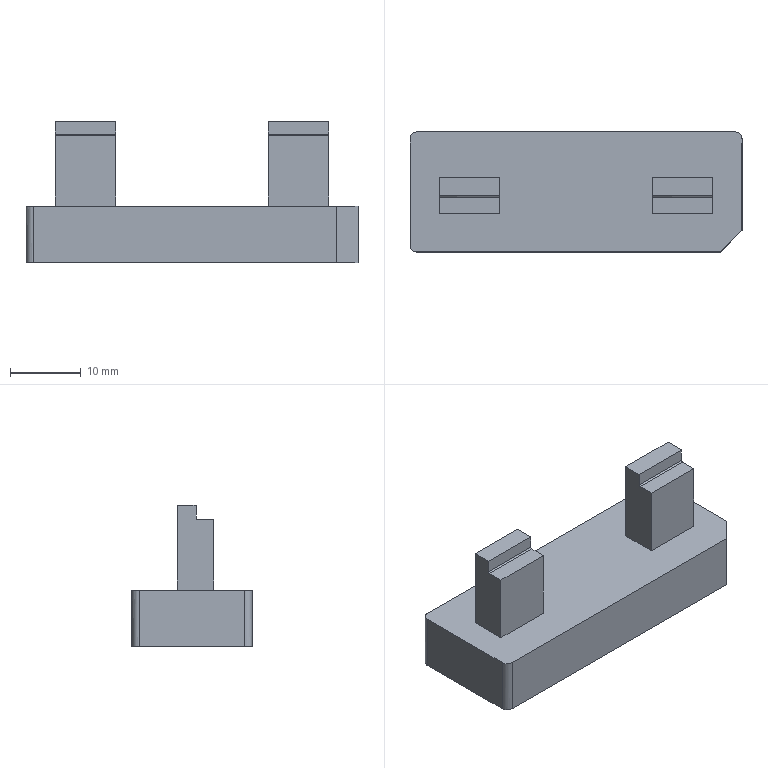NC program | PowerMill | posted by the shop | part box 47 x 17 x 19.985 mm
Lines 11899 to 13567 of 62704:
( TOOL ID   D4_2 )
( TOOL DIA. 4. TIP RAD 0 LENGTH 67.16 )
( Z = -12.15 )
T14 M6
T13
G91 G28 Z0
G0 G90 G54
M08
S18000 M3
X0 Y0 M8
G43 Z10.805 H14
X15.705 Y-3.15
Z.909
G1 Z-.291 F1200
X15.703 Y-3.099 F2000
X15.698 Y-3.049
X15.688 Y-2.999
X15.674 Y-2.951
X15.656 Y-2.903
X15.635 Y-2.858
X15.61 Y-2.814
X15.582 Y-2.772
X15.55 Y-2.732
X15.516 Y-2.695
X15.479 Y-2.661
X15.439 Y-2.63
X15.397 Y-2.602
X15.353 Y-2.578
X15.307 Y-2.557
X15.259 Y-2.54
X15.21 Y-2.526
X15.161 Y-2.517
X15.11 Y-2.511
X15.065 Y-2.51
X12.484
X11.06
X10.909
X10.834 Y-2.509
X10.759 Y-2.507
X10.682 Y-2.503
X10.6 Y-2.496
X10.517 Y-2.485
X10.442 Y-2.471
X10.369 Y-2.455
X10.296 Y-2.436
X10.214 Y-2.41
X10.132 Y-2.38
X10.051 Y-2.347
X9.971 Y-2.309
X9.892 Y-2.268
X9.817 Y-2.224
X9.743 Y-2.177
X9.672 Y-2.126
X9.603 Y-2.072
X9.537 Y-2.015
X9.473 Y-1.956
X9.413 Y-1.893
X9.355 Y-1.827
X9.3 Y-1.759
X9.248 Y-1.688
X9.199 Y-1.616
X9.154 Y-1.541
X9.112 Y-1.463
X9.074 Y-1.384
X9.039 Y-1.303
X9.008 Y-1.221
X8.981 Y-1.138
X8.96 Y-1.06
X8.941 Y-.982
X8.927 Y-.903
X8.916 Y-.822
X8.907 Y-.735
X8.902 Y-.641
X8.9 Y-.54
Y-.438
Y.398
Y1.328
X8.899 Y1.915
Y2.02
X8.9 Y2.126
X8.905 Y2.222
X8.913 Y2.312
X8.924 Y2.396
X8.938 Y2.476
X8.956 Y2.555
X8.979 Y2.639
X9.006 Y2.723
X9.037 Y2.806
X9.071 Y2.886
X9.109 Y2.965
X9.15 Y3.042
X9.195 Y3.117
X9.243 Y3.19
X9.295 Y3.261
X9.35 Y3.329
X9.408 Y3.395
X9.469 Y3.458
X9.532 Y3.519
X9.599 Y3.576
X9.667 Y3.631
X9.739 Y3.682
X9.812 Y3.729
X9.887 Y3.773
X9.964 Y3.814
X10.043 Y3.851
X10.124 Y3.885
X10.207 Y3.915
X10.291 Y3.942
X10.376 Y3.964
X10.449 Y3.98
X10.523 Y3.994
X10.596 Y4.004
X10.67 Y4.011
X10.755 Y4.015
X10.839 Y4.017
X10.914
X15.116
X19.221 Y4.018
X19.294 Y4.017
X19.396 Y4.016
X19.48 Y4.011
X19.554 Y4.004
X19.625 Y3.994
X19.714 Y3.978
X19.8 Y3.958
X19.884 Y3.934
X19.967 Y3.907
X20.049 Y3.876
X20.129 Y3.842
X20.208 Y3.803
X20.284 Y3.761
X20.359 Y3.716
X20.432 Y3.667
X20.503 Y3.615
X20.571 Y3.56
X20.637 Y3.501
X20.7 Y3.44
X20.759 Y3.376
X20.816 Y3.31
X20.87 Y3.24
X20.921 Y3.169
X20.968 Y3.095
X21.012 Y3.019
X21.053 Y2.941
X21.089 Y2.862
X21.123 Y2.781
X21.152 Y2.698
X21.178 Y2.614
X21.198 Y2.538
X21.214 Y2.461
X21.227 Y2.383
X21.238 Y2.3
X21.245 Y2.21
X21.249 Y2.12
X21.25 Y2.033
Y1.944
Y.971
Y.173
Y-.287
X21.251 Y-.519
X21.25 Y-.62
X21.245 Y-.715
X21.237 Y-.804
X21.226 Y-.89
X21.211 Y-.971
X21.193 Y-1.052
X21.169 Y-1.136
X21.142 Y-1.22
X21.111 Y-1.302
X21.077 Y-1.383
X21.038 Y-1.462
X20.997 Y-1.539
X20.951 Y-1.614
X20.903 Y-1.687
X20.851 Y-1.758
X20.796 Y-1.826
X20.738 Y-1.892
X20.677 Y-1.955
X20.613 Y-2.015
X20.547 Y-2.072
X20.478 Y-2.126
X20.406 Y-2.177
X20.333 Y-2.225
X20.257 Y-2.269
X20.179 Y-2.31
X20.1 Y-2.347
X20.019 Y-2.38
X19.936 Y-2.41
X19.852 Y-2.436
X19.768 Y-2.458
X19.682 Y-2.476
X19.65 Y-2.482
X19.565 Y-2.495
X19.477 Y-2.504
X19.398 Y-2.508
X19.319 Y-2.51
X19.24
X19.161
X15.065
X15.015 Y-2.512
X14.965 Y-2.518
X14.915 Y-2.528
X14.867 Y-2.541
X14.819 Y-2.559
X14.773 Y-2.58
X14.729 Y-2.605
X14.687 Y-2.633
X14.648 Y-2.665
X14.611 Y-2.699
X14.577 Y-2.736
X14.546 Y-2.776
X14.518 Y-2.818
X14.493 Y-2.863
X14.473 Y-2.909
X14.455 Y-2.956
X14.442 Y-3.005
X14.433 Y-3.055
X14.427 Y-3.105
X14.425 Y-3.15
X15.705 Z-.391
X15.703 Y-3.099
X15.698 Y-3.049
X15.688 Y-2.999
X15.674 Y-2.951
X15.656 Y-2.903
X15.635 Y-2.858
X15.61 Y-2.814
X15.582 Y-2.772
X15.55 Y-2.732
X15.516 Y-2.695
X15.479 Y-2.661
X15.439 Y-2.63
X15.397 Y-2.602
X15.353 Y-2.578
X15.307 Y-2.557
X15.259 Y-2.54
X15.21 Y-2.526
X15.161 Y-2.517
X15.11 Y-2.511
X15.065 Y-2.51
X12.484
X11.06
X10.909
X10.834 Y-2.509
X10.759 Y-2.507
X10.682 Y-2.503
X10.6 Y-2.496
X10.517 Y-2.485
X10.442 Y-2.471
X10.369 Y-2.455
X10.296 Y-2.436
X10.214 Y-2.41
X10.132 Y-2.38
X10.051 Y-2.347
X9.971 Y-2.309
X9.892 Y-2.268
X9.817 Y-2.224
X9.743 Y-2.177
X9.672 Y-2.126
X9.603 Y-2.072
X9.537 Y-2.015
X9.473 Y-1.956
X9.413 Y-1.893
X9.355 Y-1.827
X9.3 Y-1.759
X9.248 Y-1.688
X9.199 Y-1.616
X9.154 Y-1.541
X9.112 Y-1.463
X9.074 Y-1.384
X9.039 Y-1.303
X9.008 Y-1.221
X8.981 Y-1.138
X8.96 Y-1.06
X8.941 Y-.982
X8.927 Y-.903
X8.916 Y-.822
X8.907 Y-.735
X8.902 Y-.641
X8.9 Y-.54
Y-.438
Y.397
Y1.328
Y1.786
X8.899 Y2.02
X8.9 Y2.123
X8.905 Y2.218
X8.912 Y2.308
X8.924 Y2.393
X8.938 Y2.474
X8.956 Y2.554
X8.979 Y2.638
X9.006 Y2.722
X9.037 Y2.805
X9.071 Y2.885
X9.109 Y2.964
X9.15 Y3.041
X9.195 Y3.116
X9.243 Y3.189
X9.294 Y3.26
X9.349 Y3.328
X9.407 Y3.394
X9.468 Y3.458
X9.532 Y3.518
X9.598 Y3.576
X9.667 Y3.63
X9.738 Y3.681
X9.811 Y3.729
X9.886 Y3.773
X9.963 Y3.814
X10.042 Y3.851
X10.123 Y3.884
X10.206 Y3.915
X10.291 Y3.941
X10.375 Y3.964
X10.448 Y3.98
X10.522 Y3.994
X10.595 Y4.004
X10.67 Y4.011
X10.754 Y4.015
X10.838 Y4.017
X10.913
X15.114
X19.221 Y4.018
X19.294 Y4.017
X19.396 Y4.016
X19.48 Y4.011
X19.554 Y4.004
X19.625 Y3.994
X19.714 Y3.978
X19.8 Y3.958
X19.884 Y3.934
X19.967 Y3.907
X20.049 Y3.876
X20.129 Y3.842
X20.208 Y3.803
X20.284 Y3.761
X20.359 Y3.716
X20.432 Y3.667
X20.503 Y3.615
X20.571 Y3.56
X20.637 Y3.501
X20.7 Y3.44
X20.759 Y3.376
X20.816 Y3.31
X20.87 Y3.24
X20.921 Y3.169
X20.968 Y3.095
X21.012 Y3.019
X21.053 Y2.941
X21.089 Y2.862
X21.123 Y2.781
X21.152 Y2.698
X21.178 Y2.614
X21.198 Y2.538
X21.214 Y2.461
X21.227 Y2.383
X21.238 Y2.3
X21.245 Y2.21
X21.249 Y2.12
X21.25 Y2.033
Y1.944
Y.971
Y.173
Y-.287
X21.251 Y-.519
X21.25 Y-.62
X21.245 Y-.715
X21.237 Y-.804
X21.226 Y-.89
X21.211 Y-.971
X21.193 Y-1.052
X21.169 Y-1.136
X21.142 Y-1.22
X21.111 Y-1.302
X21.076 Y-1.383
X21.038 Y-1.462
X20.997 Y-1.539
X20.952 Y-1.614
X20.903 Y-1.687
X20.851 Y-1.758
X20.796 Y-1.826
X20.738 Y-1.892
X20.677 Y-1.955
X20.613 Y-2.015
X20.547 Y-2.072
X20.478 Y-2.126
X20.407 Y-2.177
X20.333 Y-2.225
X20.257 Y-2.269
X20.18 Y-2.309
X20.1 Y-2.347
X20.019 Y-2.38
X19.936 Y-2.41
X19.852 Y-2.436
X19.767 Y-2.458
X19.681 Y-2.477
X19.65 Y-2.482
X19.622 Y-2.487
X19.593 Y-2.49
X19.559 Y-2.495
X19.53 Y-2.498
X19.502 Y-2.501
X19.473 Y-2.504
X19.445 Y-2.506
X19.353 Y-2.509
X19.26 Y-2.51
X19.168
X15.065
X15.015 Y-2.512
X14.965 Y-2.518
X14.915 Y-2.528
X14.867 Y-2.541
X14.819 Y-2.559
X14.773 Y-2.58
X14.729 Y-2.605
X14.687 Y-2.633
X14.648 Y-2.665
X14.611 Y-2.699
X14.577 Y-2.736
X14.546 Y-2.776
X14.518 Y-2.818
X14.493 Y-2.863
X14.473 Y-2.909
X14.455 Y-2.956
X14.442 Y-3.005
X14.433 Y-3.055
X14.427 Y-3.105
X14.425 Y-3.15
X15.705 Z-.491
X15.703 Y-3.099
X15.698 Y-3.049
X15.688 Y-2.999
X15.674 Y-2.951
X15.656 Y-2.903
X15.635 Y-2.858
X15.61 Y-2.814
X15.582 Y-2.772
X15.55 Y-2.732
X15.516 Y-2.695
X15.479 Y-2.661
X15.439 Y-2.63
X15.397 Y-2.602
X15.353 Y-2.578
X15.307 Y-2.557
X15.259 Y-2.54
X15.21 Y-2.526
X15.161 Y-2.517
X15.11 Y-2.511
X15.065 Y-2.51
X12.484
X11.06
X10.909
X10.834 Y-2.509
X10.759 Y-2.507
X10.682 Y-2.503
X10.6 Y-2.496
X10.517 Y-2.485
X10.442 Y-2.471
X10.369 Y-2.455
X10.296 Y-2.436
X10.214 Y-2.41
X10.132 Y-2.38
X10.051 Y-2.347
X9.971 Y-2.309
X9.892 Y-2.268
X9.817 Y-2.224
X9.743 Y-2.177
X9.672 Y-2.126
X9.603 Y-2.072
X9.537 Y-2.015
X9.473 Y-1.956
X9.413 Y-1.893
X9.355 Y-1.827
X9.3 Y-1.759
X9.248 Y-1.688
X9.199 Y-1.616
X9.154 Y-1.541
X9.112 Y-1.463
X9.074 Y-1.384
X9.039 Y-1.303
X9.008 Y-1.221
X8.981 Y-1.138
X8.96 Y-1.06
X8.941 Y-.982
X8.927 Y-.903
X8.916 Y-.822
X8.907 Y-.735
X8.902 Y-.641
X8.9 Y-.54
Y-.438
Y.397
Y1.328
Y1.786
X8.899 Y2.02
X8.9 Y2.123
X8.905 Y2.218
X8.912 Y2.308
X8.924 Y2.393
X8.938 Y2.474
X8.956 Y2.554
X8.979 Y2.638
X9.006 Y2.722
X9.037 Y2.805
X9.071 Y2.885
X9.109 Y2.964
X9.15 Y3.041
X9.195 Y3.116
X9.243 Y3.189
X9.294 Y3.26
X9.349 Y3.328
X9.407 Y3.394
X9.468 Y3.458
X9.532 Y3.518
X9.598 Y3.576
X9.667 Y3.63
X9.738 Y3.681
X9.811 Y3.729
X9.886 Y3.773
X9.963 Y3.814
X10.042 Y3.851
X10.123 Y3.884
X10.206 Y3.915
X10.291 Y3.941
X10.375 Y3.964
X10.448 Y3.98
X10.522 Y3.994
X10.595 Y4.004
X10.67 Y4.011
X10.754 Y4.015
X10.838 Y4.017
X10.913
X15.114
X19.221 Y4.018
X19.294 Y4.017
X19.396 Y4.016
X19.48 Y4.011
X19.554 Y4.004
X19.625 Y3.994
X19.714 Y3.978
X19.8 Y3.958
X19.884 Y3.934
X19.967 Y3.907
X20.049 Y3.876
X20.129 Y3.842
X20.208 Y3.803
X20.284 Y3.761
X20.359 Y3.716
X20.432 Y3.667
X20.503 Y3.615
X20.571 Y3.56
X20.637 Y3.501
X20.7 Y3.44
X20.759 Y3.376
X20.816 Y3.31
X20.87 Y3.24
X20.921 Y3.169
X20.968 Y3.095
X21.012 Y3.019
X21.053 Y2.941
X21.089 Y2.862
X21.123 Y2.781
X21.152 Y2.698
X21.178 Y2.614
X21.198 Y2.538
X21.214 Y2.461
X21.227 Y2.383
X21.238 Y2.3
X21.245 Y2.21
X21.249 Y2.12
X21.25 Y2.033
Y1.944
Y.971
Y.068
X21.251 Y-.497
Y-.585
X21.248 Y-.675
X21.241 Y-.765
X21.232 Y-.851
X21.218 Y-.932
X21.202 Y-1.012
X21.182 Y-1.09
X21.157 Y-1.174
X21.129 Y-1.257
X21.096 Y-1.339
X21.06 Y-1.418
X21.02 Y-1.497
X20.977 Y-1.573
X20.93 Y-1.647
X20.88 Y-1.719
X20.827 Y-1.789
X20.771 Y-1.856
X20.711 Y-1.92
X20.649 Y-1.982
X20.584 Y-2.041
X20.516 Y-2.097
X20.446 Y-2.149
X20.374 Y-2.199
X20.299 Y-2.245
X20.222 Y-2.288
X20.144 Y-2.327
X20.064 Y-2.362
X19.982 Y-2.394
X19.899 Y-2.422
X19.815 Y-2.446
X19.729 Y-2.467
X19.65 Y-2.482
X19.565 Y-2.495
X19.477 Y-2.504
X19.398 Y-2.508
X19.319 Y-2.51
X19.24
X19.161
X15.065
X15.015 Y-2.512
X14.965 Y-2.518
X14.915 Y-2.528
X14.867 Y-2.541
X14.819 Y-2.559
X14.773 Y-2.58
X14.729 Y-2.605
X14.687 Y-2.633
X14.648 Y-2.665
X14.611 Y-2.699
X14.577 Y-2.736
X14.546 Y-2.776
X14.518 Y-2.818
X14.493 Y-2.863
X14.473 Y-2.909
X14.455 Y-2.956
X14.442 Y-3.005
X14.433 Y-3.055
X14.427 Y-3.105
X14.425 Y-3.15
X15.705 Z-.59
X15.703 Y-3.099
X15.698 Y-3.049
X15.688 Y-2.999
X15.674 Y-2.951
X15.656 Y-2.903
X15.635 Y-2.858
X15.61 Y-2.814
X15.582 Y-2.772
X15.55 Y-2.732
X15.516 Y-2.695
X15.479 Y-2.661
X15.439 Y-2.63
X15.397 Y-2.602
X15.353 Y-2.578
X15.307 Y-2.557
X15.259 Y-2.54
X15.21 Y-2.526
X15.161 Y-2.517
X15.11 Y-2.511
X15.065 Y-2.51
X12.484
X11.06
X10.909
X10.834 Y-2.509
X10.759 Y-2.507
X10.682 Y-2.503
X10.6 Y-2.496
X10.517 Y-2.485
X10.442 Y-2.471
X10.369 Y-2.455
X10.296 Y-2.436
X10.214 Y-2.41
X10.132 Y-2.38
X10.051 Y-2.347
X9.971 Y-2.309
X9.892 Y-2.268
X9.817 Y-2.224
X9.743 Y-2.177
X9.672 Y-2.126
X9.603 Y-2.072
X9.537 Y-2.015
X9.473 Y-1.956
X9.413 Y-1.893
X9.355 Y-1.827
X9.3 Y-1.759
X9.248 Y-1.688
X9.2 Y-1.616
X9.154 Y-1.541
X9.112 Y-1.463
X9.074 Y-1.384
X9.039 Y-1.303
X9.008 Y-1.221
X8.981 Y-1.138
X8.96 Y-1.06
X8.941 Y-.982
X8.927 Y-.903
X8.916 Y-.822
X8.907 Y-.735
X8.902 Y-.641
X8.9 Y-.54
Y-.438
Y.397
Y1.328
Y1.786
X8.899 Y2.02
X8.9 Y2.123
X8.905 Y2.218
X8.912 Y2.308
X8.924 Y2.393
X8.938 Y2.474
X8.956 Y2.554
X8.979 Y2.638
X9.006 Y2.722
X9.037 Y2.805
X9.071 Y2.885
X9.109 Y2.964
X9.15 Y3.041
X9.195 Y3.116
X9.243 Y3.189
X9.294 Y3.26
X9.349 Y3.328
X9.407 Y3.394
X9.468 Y3.458
X9.532 Y3.518
X9.598 Y3.576
X9.667 Y3.63
X9.738 Y3.681
X9.811 Y3.729
X9.886 Y3.773
X9.963 Y3.814
X10.042 Y3.851
X10.123 Y3.884
X10.206 Y3.915
X10.291 Y3.941
X10.375 Y3.964
X10.448 Y3.98
X10.522 Y3.994
X10.595 Y4.004
X10.67 Y4.011
X10.754 Y4.015
X10.838 Y4.017
X10.913
X15.114
X19.221 Y4.018
X19.294 Y4.017
X19.396 Y4.016
X19.48 Y4.011
X19.554 Y4.004
X19.625 Y3.994
X19.714 Y3.978
X19.8 Y3.958
X19.884 Y3.934
X19.967 Y3.907
X20.049 Y3.876
X20.129 Y3.842
X20.208 Y3.803
X20.284 Y3.761
X20.359 Y3.716
X20.432 Y3.667
X20.503 Y3.615
X20.571 Y3.56
X20.637 Y3.501
X20.7 Y3.44
X20.759 Y3.376
X20.816 Y3.31
X20.87 Y3.24
X20.921 Y3.169
X20.968 Y3.095
X21.012 Y3.019
X21.053 Y2.941
X21.089 Y2.862
X21.123 Y2.781
X21.152 Y2.698
X21.178 Y2.614
X21.198 Y2.538
X21.214 Y2.461
X21.227 Y2.383
X21.238 Y2.3
X21.245 Y2.21
X21.249 Y2.12
X21.25 Y2.033
Y1.944
Y.971
Y.074
X21.251 Y-.486
Y-.575
X21.248 Y-.665
X21.242 Y-.755
X21.232 Y-.842
X21.219 Y-.925
X21.203 Y-1.005
X21.184 Y-1.085
X21.161 Y-1.163
X21.133 Y-1.246
X21.101 Y-1.328
X21.065 Y-1.408
X21.026 Y-1.486
X20.983 Y-1.562
X20.937 Y-1.637
X20.887 Y-1.709
X20.835 Y-1.779
X20.779 Y-1.847
X20.72 Y-1.911
X20.658 Y-1.973
X20.593 Y-2.033
X20.526 Y-2.089
X20.456 Y-2.142
X20.384 Y-2.192
X20.31 Y-2.238
X20.235 Y-2.281
X20.157 Y-2.32
X20.078 Y-2.356
X19.996 Y-2.389
X19.913 Y-2.418
X19.831 Y-2.442
X19.749 Y-2.463
X19.667 Y-2.479
X19.65 Y-2.482
X19.558 Y-2.495
X19.471 Y-2.504
X19.393 Y-2.508
X19.314 Y-2.51
X19.236
X19.158
X15.065
X15.015 Y-2.512
X14.965 Y-2.518
X14.915 Y-2.528
X14.867 Y-2.541
X14.819 Y-2.559
X14.773 Y-2.58
X14.729 Y-2.605
X14.687 Y-2.633
X14.648 Y-2.665
X14.611 Y-2.699
X14.577 Y-2.736
X14.546 Y-2.776
X14.518 Y-2.818
X14.493 Y-2.863
X14.473 Y-2.909
X14.455 Y-2.956
X14.442 Y-3.005
X14.433 Y-3.055
X14.427 Y-3.105
X14.425 Y-3.15
X15.705 Z-.69
X15.703 Y-3.099
X15.698 Y-3.049
X15.688 Y-2.999
X15.674 Y-2.951
X15.656 Y-2.903
X15.635 Y-2.858
X15.61 Y-2.814
X15.582 Y-2.772
X15.55 Y-2.732
X15.516 Y-2.695
X15.479 Y-2.661
X15.439 Y-2.63
X15.397 Y-2.602
X15.353 Y-2.578
X15.307 Y-2.557
X15.259 Y-2.54
X15.21 Y-2.526
X15.161 Y-2.517
X15.11 Y-2.511
X15.065 Y-2.51
X12.484
X11.06
X10.909
X10.834 Y-2.509
X10.759 Y-2.507
X10.682 Y-2.503
X10.6 Y-2.496
X10.517 Y-2.485
X10.442 Y-2.471
X10.369 Y-2.455
X10.296 Y-2.436
X10.214 Y-2.41
X10.132 Y-2.38
X10.051 Y-2.347
X9.971 Y-2.309
X9.892 Y-2.268
X9.817 Y-2.224
X9.743 Y-2.177
X9.672 Y-2.126
X9.603 Y-2.072
X9.537 Y-2.015
X9.473 Y-1.956
X9.413 Y-1.893
X9.355 Y-1.827
X9.3 Y-1.759
X9.248 Y-1.688
X9.2 Y-1.616
X9.154 Y-1.541
X9.112 Y-1.463
X9.074 Y-1.384
X9.039 Y-1.303
X9.008 Y-1.221
X8.981 Y-1.138
X8.96 Y-1.06
X8.941 Y-.982
X8.927 Y-.903
X8.916 Y-.822
X8.907 Y-.735
X8.902 Y-.641
X8.9 Y-.54
Y-.438
Y.397
Y1.328
Y1.786
X8.899 Y2.02
X8.9 Y2.123
X8.905 Y2.218
X8.912 Y2.308
X8.924 Y2.393
X8.938 Y2.474
X8.956 Y2.554
X8.979 Y2.638
X9.006 Y2.722
X9.037 Y2.805
X9.071 Y2.885
X9.109 Y2.964
X9.15 Y3.041
X9.195 Y3.116
X9.243 Y3.189
X9.294 Y3.26
X9.349 Y3.328
X9.407 Y3.394
X9.468 Y3.458
X9.532 Y3.518
X9.598 Y3.576
X9.667 Y3.63
X9.738 Y3.681
X9.811 Y3.729
X9.886 Y3.773
X9.963 Y3.814
X10.042 Y3.851
X10.123 Y3.884
X10.206 Y3.915
X10.291 Y3.941
X10.375 Y3.964
X10.448 Y3.98
X10.522 Y3.994
X10.595 Y4.004
X10.67 Y4.011
X10.754 Y4.015
X10.838 Y4.017
X10.913
X15.114
X19.221 Y4.018
X19.294 Y4.017
X19.396 Y4.016
X19.48 Y4.011
X19.554 Y4.004
X19.625 Y3.994
X19.714 Y3.978
X19.8 Y3.958
X19.884 Y3.934
X19.967 Y3.907
X20.049 Y3.876
X20.129 Y3.842
X20.208 Y3.803
X20.284 Y3.761
X20.359 Y3.716
X20.432 Y3.667
X20.503 Y3.615
X20.571 Y3.56
X20.637 Y3.501
X20.7 Y3.44
X20.759 Y3.376
X20.816 Y3.31
X20.87 Y3.24
X20.921 Y3.169
X20.968 Y3.095
X21.012 Y3.019
X21.053 Y2.941
X21.089 Y2.862
X21.123 Y2.781
X21.152 Y2.698
X21.178 Y2.614
X21.198 Y2.538
X21.214 Y2.461
X21.227 Y2.383
X21.238 Y2.3
X21.245 Y2.21
X21.249 Y2.12
X21.25 Y2.033
Y1.944
Y.971
Y.069
X21.251 Y-.496
Y-.585
X21.248 Y-.674
X21.241 Y-.764
X21.232 Y-.85
X21.218 Y-.932
X21.202 Y-1.011
X21.182 Y-1.09
X21.158 Y-1.174
X21.129 Y-1.257
X21.096 Y-1.338
X21.06 Y-1.418
X21.02 Y-1.496
X20.977 Y-1.573
X20.93 Y-1.647
X20.88 Y-1.719
X20.827 Y-1.789
X20.771 Y-1.856
X20.711 Y-1.92
X20.649 Y-1.982
X20.584 Y-2.041
X20.516 Y-2.097
X20.446 Y-2.149
X20.374 Y-2.199
X20.299 Y-2.245
X20.223 Y-2.288
X20.144 Y-2.327
X20.064 Y-2.362
X19.982 Y-2.394
X19.899 Y-2.422
X19.815 Y-2.446
X19.73 Y-2.467
X19.65 Y-2.482
X19.565 Y-2.495
X19.477 Y-2.504
X19.398 Y-2.508
X19.319 Y-2.51
X19.24
X19.161
X15.065
X15.015 Y-2.512
X14.965 Y-2.518
X14.915 Y-2.528
X14.867 Y-2.541
X14.819 Y-2.559
X14.773 Y-2.58
X14.729 Y-2.605
X14.687 Y-2.633
X14.648 Y-2.665
X14.611 Y-2.699
X14.577 Y-2.736
X14.546 Y-2.776
X14.518 Y-2.818
X14.493 Y-2.863
X14.473 Y-2.909
X14.455 Y-2.956
X14.442 Y-3.005
X14.433 Y-3.055
X14.427 Y-3.105
X14.425 Y-3.15
X15.705 Z-.789
X15.703 Y-3.099
X15.698 Y-3.049
X15.688 Y-2.999
X15.674 Y-2.951
X15.656 Y-2.903
X15.635 Y-2.858
X15.61 Y-2.814
X15.582 Y-2.772
X15.55 Y-2.732
X15.516 Y-2.695
X15.479 Y-2.661
X15.439 Y-2.63
X15.397 Y-2.602
X15.353 Y-2.578
X15.307 Y-2.557
X15.259 Y-2.54
X15.21 Y-2.526
X15.161 Y-2.517
X15.11 Y-2.511
X15.065 Y-2.51
X14.374
X11.948
X10.909
X10.793 Y-2.508
X10.697 Y-2.505
X10.613 Y-2.498
X10.537 Y-2.488
X10.464 Y-2.476
X10.376 Y-2.456
X10.29 Y-2.434
X10.205 Y-2.407
X10.122 Y-2.376
X10.041 Y-2.343
X9.962 Y-2.305
X9.885 Y-2.264
X9.81 Y-2.22
X9.736 Y-2.172
X9.665 Y-2.121
X9.597 Y-2.067
X9.531 Y-2.01
X9.467 Y-1.949
X9.407 Y-1.886
X9.349 Y-1.82
X9.294 Y-1.752
X9.243 Y-1.681
X9.195 Y-1.608
X9.149 Y-1.532
X9.108 Y-1.455
X9.07 Y-1.376
X9.036 Y-1.296
X9.006 Y-1.214
X8.979 Y-1.131
X8.957 Y-1.052
X8.941 Y-.981
X8.928 Y-.91
X8.917 Y-.839
X8.908 Y-.767
X8.903 Y-.695
X8.901 Y-.622
X8.9 Y-.55
Y-.477
Y.717
Y1.328
Y1.786
X8.899 Y2.02
X8.9 Y2.123
X8.905 Y2.218
X8.912 Y2.308
X8.924 Y2.393
X8.938 Y2.474
X8.956 Y2.554
X8.979 Y2.638
X9.006 Y2.722
X9.037 Y2.805
X9.071 Y2.885
X9.109 Y2.964
X9.15 Y3.041
X9.195 Y3.116
X9.243 Y3.189
X9.294 Y3.26
X9.349 Y3.328
X9.407 Y3.394
X9.468 Y3.458
X9.532 Y3.518
X9.598 Y3.576
X9.667 Y3.63
X9.738 Y3.681
X9.811 Y3.729
X9.886 Y3.773
X9.963 Y3.814
X10.042 Y3.851
X10.123 Y3.884
X10.206 Y3.915
X10.291 Y3.941
X10.375 Y3.964
X10.448 Y3.98
X10.522 Y3.994
X10.595 Y4.004
X10.67 Y4.011
X10.754 Y4.015
X10.838 Y4.017
X10.913
X15.114
X19.221 Y4.018
X19.294 Y4.017
X19.396 Y4.016
X19.48 Y4.011
X19.554 Y4.004
X19.625 Y3.994
X19.714 Y3.978
X19.8 Y3.958
X19.884 Y3.934
X19.967 Y3.907
X20.049 Y3.876
X20.129 Y3.842
X20.208 Y3.803
X20.284 Y3.761
X20.359 Y3.716
X20.432 Y3.667
X20.503 Y3.615
X20.571 Y3.56
X20.637 Y3.501
X20.7 Y3.44
X20.759 Y3.376
X20.816 Y3.31
X20.87 Y3.24
X20.921 Y3.169
X20.968 Y3.095
X21.012 Y3.019
X21.053 Y2.941
X21.089 Y2.862
X21.123 Y2.781
X21.152 Y2.698
X21.178 Y2.614
X21.198 Y2.538
X21.214 Y2.461
X21.227 Y2.383
X21.238 Y2.3
X21.245 Y2.21
X21.249 Y2.12
X21.25 Y2.033
Y1.944
Y.971
Y.173
Y-.407
Y-.519
X21.249 Y-.61
X21.245 Y-.703
X21.238 Y-.792
X21.228 Y-.876
X21.214 Y-.954
X21.198 Y-1.032
X21.178 Y-1.108
X21.152 Y-1.193
X21.122 Y-1.275
X21.088 Y-1.357
X21.051 Y-1.437
X21.01 Y-1.515
X20.966 Y-1.591
X20.919 Y-1.664
X20.868 Y-1.736
X20.814 Y-1.805
X20.757 Y-1.871
X20.697 Y-1.935
X20.634 Y-1.996
X20.569 Y-2.054
X20.501 Y-2.109
X20.43 Y-2.161
X20.357 Y-2.21
X20.282 Y-2.255
X20.205 Y-2.297
X20.126 Y-2.335
X20.045 Y-2.37
X19.963 Y-2.401
X19.88 Y-2.428
X19.796 Y-2.451
X19.71 Y-2.471
X19.65 Y-2.482
X19.565 Y-2.495
X19.477 Y-2.504
X19.398 Y-2.508
X19.319 Y-2.51
X19.239
X19.16
X15.065
X15.015 Y-2.512
X14.965 Y-2.518
X14.915 Y-2.528
X14.867 Y-2.541
X14.819 Y-2.559
X14.773 Y-2.58
X14.729 Y-2.605
X14.687 Y-2.633
X14.648 Y-2.665
X14.611 Y-2.699
X14.577 Y-2.736
X14.546 Y-2.776
X14.518 Y-2.818
X14.493 Y-2.863
X14.473 Y-2.909
X14.455 Y-2.956
X14.442 Y-3.005
X14.433 Y-3.055
X14.427 Y-3.105
X14.425 Y-3.15
X15.705 Z-.889
X15.703 Y-3.099
X15.698 Y-3.049
X15.688 Y-2.999
X15.674 Y-2.951
X15.656 Y-2.903
X15.635 Y-2.858
X15.61 Y-2.814
X15.582 Y-2.772
X15.55 Y-2.732
X15.516 Y-2.695
X15.479 Y-2.661
X15.439 Y-2.63
X15.397 Y-2.602
X15.353 Y-2.578
X15.307 Y-2.557
X15.259 Y-2.54
X15.21 Y-2.526
X15.161 Y-2.517
X15.11 Y-2.511
X15.065 Y-2.51
X12.484
X11.06
X10.909
X10.834 Y-2.509
X10.759 Y-2.507
X10.682 Y-2.503
X10.6 Y-2.496
X10.517 Y-2.485
X10.442 Y-2.471
X10.369 Y-2.455
X10.296 Y-2.436
X10.214 Y-2.41
X10.132 Y-2.38
X10.051 Y-2.347
X9.971 Y-2.309
X9.892 Y-2.268
X9.817 Y-2.224
X9.743 Y-2.177
X9.672 Y-2.126
X9.603 Y-2.072
X9.537 Y-2.015
X9.473 Y-1.956
X9.413 Y-1.893
X9.355 Y-1.827
X9.3 Y-1.759
X9.248 Y-1.688
X9.199 Y-1.616
X9.154 Y-1.541
X9.112 Y-1.463
X9.074 Y-1.384
X9.039 Y-1.303
X9.008 Y-1.221
X8.981 Y-1.138
X8.96 Y-1.06
X8.941 Y-.982
X8.927 Y-.904
X8.916 Y-.822
X8.907 Y-.735
X8.902 Y-.641
X8.9 Y-.54
Y-.438
Y.397
Y1.328
Y1.786
X8.899 Y2.02
X8.9 Y2.123
X8.905 Y2.218
X8.912 Y2.308
X8.924 Y2.393
X8.938 Y2.474
X8.956 Y2.554
X8.979 Y2.638
X9.006 Y2.722
X9.037 Y2.805
X9.071 Y2.885
X9.109 Y2.964
X9.15 Y3.041
X9.195 Y3.116
X9.243 Y3.189
X9.294 Y3.26
X9.349 Y3.328
X9.407 Y3.394
X9.468 Y3.458
X9.532 Y3.518
X9.598 Y3.576
X9.667 Y3.63
X9.738 Y3.681
X9.811 Y3.729
X9.886 Y3.773
X9.963 Y3.814
X10.042 Y3.851
X10.123 Y3.884
X10.206 Y3.915
X10.291 Y3.941
X10.375 Y3.964
X10.448 Y3.98
X10.522 Y3.994
X10.595 Y4.004
X10.67 Y4.011
X10.754 Y4.015
X10.838 Y4.017
X10.913
X15.114
X19.221 Y4.018
X19.294 Y4.017
X19.396 Y4.016
X19.48 Y4.011
X19.554 Y4.004
X19.625 Y3.994
X19.714 Y3.978
X19.8 Y3.958
X19.884 Y3.934
X19.967 Y3.907
X20.049 Y3.876
X20.129 Y3.842
X20.208 Y3.803
X20.284 Y3.761
X20.359 Y3.716
X20.432 Y3.667
X20.503 Y3.615
X20.571 Y3.56
X20.637 Y3.501
X20.7 Y3.44
X20.759 Y3.376
X20.816 Y3.31
X20.87 Y3.24
X20.921 Y3.169
X20.968 Y3.095
X21.012 Y3.019
X21.053 Y2.941
X21.089 Y2.862
X21.123 Y2.781
X21.152 Y2.698
X21.178 Y2.614
X21.198 Y2.538
X21.214 Y2.461
X21.227 Y2.383
X21.238 Y2.3
X21.245 Y2.21
X21.249 Y2.12
X21.25 Y2.033
Y1.944
Y.971
Y.173
Y-.407
Y-.519
X21.249 Y-.61
X21.245 Y-.703
X21.238 Y-.792
X21.228 Y-.876
X21.214 Y-.954
X21.198 Y-1.032
X21.178 Y-1.108
X21.152 Y-1.193
X21.122 Y-1.275
X21.088 Y-1.357
X21.051 Y-1.437
X21.01 Y-1.515
X20.966 Y-1.591
X20.919 Y-1.664
X20.868 Y-1.736
X20.814 Y-1.805
X20.757 Y-1.871
X20.697 Y-1.935
X20.634 Y-1.996
X20.569 Y-2.054
X20.501 Y-2.109
X20.43 Y-2.161
X20.357 Y-2.21
X20.282 Y-2.255
X20.205 Y-2.297
X20.126 Y-2.335
X20.045 Y-2.37
X19.963 Y-2.401
X19.88 Y-2.428
X19.796 Y-2.451
X19.71 Y-2.471
X19.65 Y-2.482
X19.565 Y-2.495
X19.477 Y-2.504
X19.398 Y-2.508
X19.319 Y-2.51
X19.239
X19.16
X15.065
X15.015 Y-2.512
X14.965 Y-2.518
X14.915 Y-2.528
X14.867 Y-2.541
X14.819 Y-2.559
X14.773 Y-2.58
X14.729 Y-2.605
X14.687 Y-2.633
X14.648 Y-2.665
X14.611 Y-2.699
X14.577 Y-2.736
X14.546 Y-2.776
X14.518 Y-2.818
X14.493 Y-2.863
X14.473 Y-2.909
X14.455 Y-2.956
X14.442 Y-3.005
X14.433 Y-3.055
X14.427 Y-3.105
X14.425 Y-3.15
X15.705 Z-.989
X15.703 Y-3.099
X15.698 Y-3.049
X15.688 Y-2.999
X15.674 Y-2.951
X15.656 Y-2.903
X15.635 Y-2.858
X15.61 Y-2.814
X15.582 Y-2.772
X15.55 Y-2.732
X15.516 Y-2.695
X15.479 Y-2.661
X15.439 Y-2.63
X15.397 Y-2.602
X15.353 Y-2.578
X15.307 Y-2.557
X15.259 Y-2.54
X15.21 Y-2.526
X15.161 Y-2.517
X15.11 Y-2.511
X15.065 Y-2.51
X14.367
X11.948
X10.909
X10.793 Y-2.508
X10.697 Y-2.505
X10.613 Y-2.498
X10.537 Y-2.488
X10.464 Y-2.476
X10.376 Y-2.456
X10.29 Y-2.434
X10.205 Y-2.407
X10.122 Y-2.376
X10.041 Y-2.343
X9.962 Y-2.305
X9.885 Y-2.264
X9.81 Y-2.22
X9.736 Y-2.172
X9.665 Y-2.121
X9.597 Y-2.067
X9.531 Y-2.01
X9.467 Y-1.949
X9.407 Y-1.886
X9.349 Y-1.82
X9.294 Y-1.752
X9.243 Y-1.681
X9.195 Y-1.608
X9.149 Y-1.532
X9.108 Y-1.455
X9.07 Y-1.376
X9.036 Y-1.296
X9.006 Y-1.214
X8.979 Y-1.131
X8.957 Y-1.052
X8.941 Y-.981
X8.928 Y-.91
X8.917 Y-.839
X8.908 Y-.767
X8.903 Y-.695
X8.901 Y-.622
X8.9 Y-.55
Y-.477
Y.717
Y1.328
Y1.786
X8.899 Y2.02
X8.9 Y2.123
X8.905 Y2.218
X8.912 Y2.308
X8.924 Y2.393
X8.938 Y2.474
X8.956 Y2.554
X8.979 Y2.638
X9.006 Y2.722
X9.037 Y2.805
X9.071 Y2.885
X9.109 Y2.964
X9.15 Y3.041
X9.195 Y3.116
X9.243 Y3.189
X9.294 Y3.26
X9.349 Y3.328
X9.407 Y3.394
X9.468 Y3.458
X9.532 Y3.518
X9.598 Y3.576
X9.667 Y3.63
X9.738 Y3.681
X9.811 Y3.729
X9.886 Y3.773
X9.963 Y3.814
X10.042 Y3.851
X10.123 Y3.884
X10.206 Y3.915
X10.291 Y3.941
X10.375 Y3.964
X10.448 Y3.98
X10.522 Y3.994
X10.595 Y4.004
X10.67 Y4.011
X10.754 Y4.015
X10.838 Y4.017
X10.913
X15.115
X18.182
X19.221
X19.287
X19.352 Y4.016
X19.417 Y4.014
X19.483 Y4.011
X19.553 Y4.004
X19.617 Y3.995
X19.682 Y3.984
X19.745 Y3.971
X19.83 Y3.95
X19.914 Y3.925
X19.997 Y3.896
X20.079 Y3.864
X20.158 Y3.828
X20.236 Y3.788
X20.312 Y3.745
X20.386 Y3.699
X20.458 Y3.649
X20.527 Y3.596
X20.595 Y3.539
X20.659 Y3.48
X20.721 Y3.417
X20.78 Y3.353
X20.836 Y3.285
X20.889 Y3.215
X20.938 Y3.143
X20.984 Y3.068
X21.027 Y2.992
X21.066 Y2.913
X21.102 Y2.833
X21.134 Y2.751
X21.162 Y2.668
X21.184 Y2.593
X21.203 Y2.516
X21.218 Y2.439
X21.231 Y2.36
X21.24 Y2.274
X21.246 Y2.183
X21.249 Y2.094
X21.25 Y2.007
Y1.076
Y.113
X21.251 Y-.462
Y-.551
X21.249 Y-.639
X21.244 Y-.729
X21.236 Y-.817
X21.224 Y-.901
X21.209 Y-.981
X21.19 Y-1.06
X21.168 Y-1.139
X21.141 Y-1.222
X21.11 Y-1.304
X21.076 Y-1.385
X21.038 Y-1.463
X20.996 Y-1.54
X20.951 Y-1.616
X20.902 Y-1.689
X20.85 Y-1.759
X20.795 Y-1.827
X20.737 Y-1.893
X20.676 Y-1.956
X20.612 Y-2.016
X20.546 Y-2.073
X20.477 Y-2.127
X20.405 Y-2.178
X20.332 Y-2.225
X20.257 Y-2.269
X20.18 Y-2.309
X20.101 Y-2.346
X20.019 Y-2.38
X19.936 Y-2.41
X19.854 Y-2.436
X19.772 Y-2.457
X19.69 Y-2.475
X19.65 Y-2.482
X19.558 Y-2.495
X19.471 Y-2.504
X19.393 Y-2.508
X19.314 Y-2.51
X19.236
X19.158
X15.065
X15.015 Y-2.512
X14.965 Y-2.518
X14.915 Y-2.528
X14.867 Y-2.541
X14.819 Y-2.559
X14.773 Y-2.58
X14.729 Y-2.605
X14.687 Y-2.633
X14.648 Y-2.665
X14.611 Y-2.699
X14.577 Y-2.736
X14.546 Y-2.776
X14.518 Y-2.818
X14.493 Y-2.863
X14.473 Y-2.909
X14.455 Y-2.956
X14.442 Y-3.005
X14.433 Y-3.055
X14.427 Y-3.105
X14.425 Y-3.15
X15.705 Z-1.088
X15.703 Y-3.099
X15.698 Y-3.049
X15.688 Y-2.999